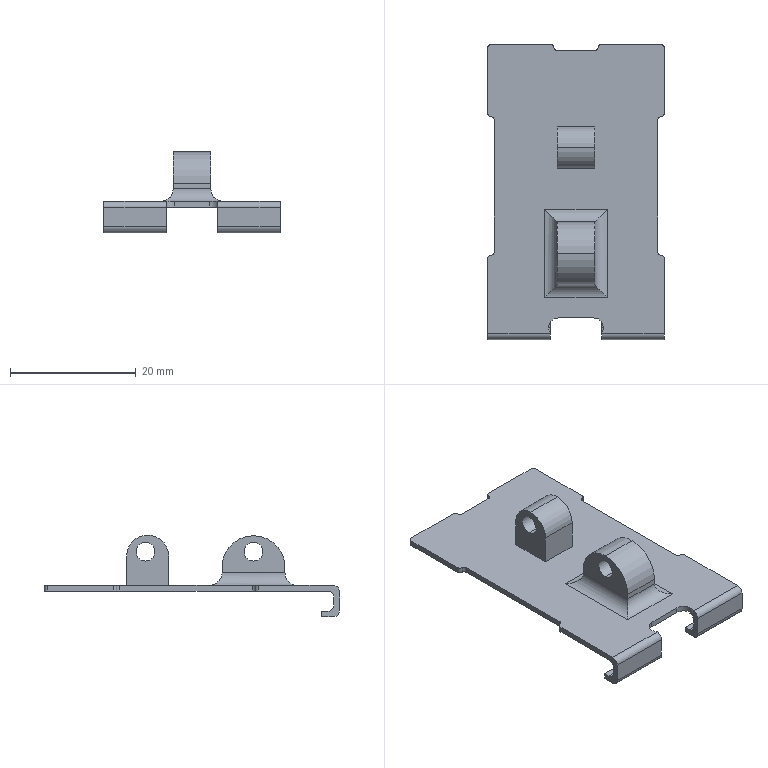Part | SolidWorks | features Fillet 6, Cut 5, ICE 3, Extrusion 1, MirrorPattern 1 | 1 solid | 71 faces | box 28 x 46.911 x 13 mm | volume 1866 mm3 | cylinder 37 | plane 34 | commonest cylinder face diameters 1 x14 2 x8 3 x4 4 x4 3.084 x3 6.667 x2